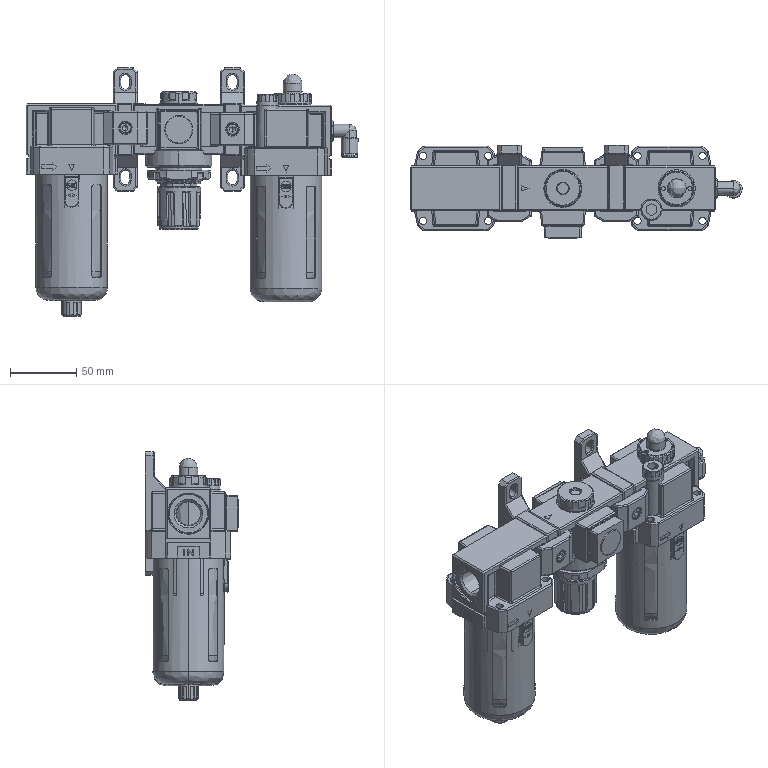Part | SolidWorks | features AEMSimFeature 1 | 15 solids | 2705 faces | box 250.3 x 70.4 x 187 mm | volume 621495 mm3 | plane 1341 | cylinder 762 | spline 308 | cone 244 | torus 45 | sphere 5 | commonest cylinder face diameters 2 x301 4 x36 5.5 x20 63.8 x16 7 x14 59 x14